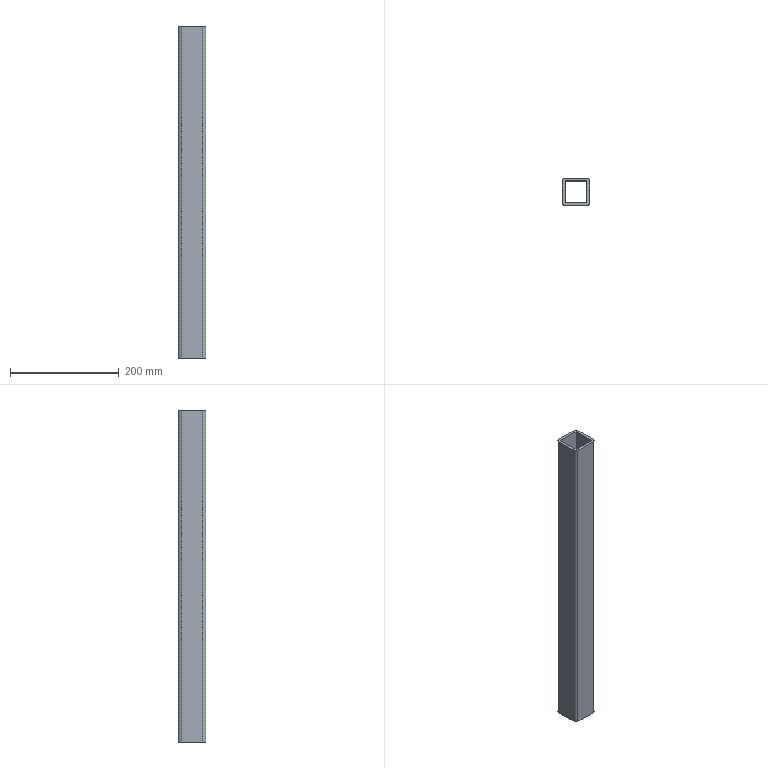Part | STEP file | SOLID | 1 solid | 14 faces | box 50 x 50 x 610 mm | volume 535909 mm3 | plane 10 | cylinder 4 | commonest cylinder face diameters 10 x4
STEP:
#1=CARTESIAN_POINT('',(0.,0.,0.));
#2=DIRECTION('',(0.,0.,1.));
#3=DIRECTION('',(1.,0.,0.));
#4=AXIS2_PLACEMENT_3D('',#1,#2,#3);
#5=CARTESIAN_POINT('',(-163.5,375.,-680.));
#6=VERTEX_POINT('',#5);
#7=CARTESIAN_POINT('',(-163.5,415.,-680.));
#8=VERTEX_POINT('',#7);
#9=CARTESIAN_POINT('',(-163.5,415.,-680.));
#10=DIRECTION('',(0.,1.,0.));
#11=VECTOR('',#10,1.);
#12=LINE('',#9,#11);
#13=CARTESIAN_POINT('',(-163.5,415.,430.));
#14=DIRECTION('',(-1.,0.,0.));
#15=DIRECTION('',(0.,1.,0.));
#16=AXIS2_PLACEMENT_3D('',#13,#14,#15);
#17=PLANE('',#16);
#18=CARTESIAN_POINT('',(0.,1110.));
#19=DIRECTION('',(1.,0.));
#20=VECTOR('',#19,1.);
#21=LINE('',#18,#20);
#22=(GEOMETRIC_REPRESENTATION_CONTEXT(2)PARAMETRIC_REPRESENTATION_CONTEXT()REPRESENTATION_CONTEXT('',''));
#23=DEFINITIONAL_REPRESENTATION('',(#21),#22);
#24=PCURVE('',#17,#23);
#25=CARTESIAN_POINT('',(-408.5,415.,-680.));
#26=DIRECTION('',(0.,0.,-1.));
#27=DIRECTION('',(0.,1.,0.));
#28=AXIS2_PLACEMENT_3D('',#25,#26,#27);
#29=PLANE('',#28);
#30=CARTESIAN_POINT('',(0.,245.));
#31=DIRECTION('',(1.,0.));
#32=VECTOR('',#31,1.);
#33=LINE('',#30,#32);
#34=(GEOMETRIC_REPRESENTATION_CONTEXT(2)PARAMETRIC_REPRESENTATION_CONTEXT()REPRESENTATION_CONTEXT('',''));
#35=DEFINITIONAL_REPRESENTATION('',(#33),#34);
#36=PCURVE('',#29,#35);
#37=SURFACE_CURVE('',#12,(#24,#36),.PCURVE_S1.);
#38=EDGE_CURVE('',#6,#8,#37,.T.);
#39=ORIENTED_EDGE('',*,*,#38,.F.);
#40=CARTESIAN_POINT('',(-163.5,375.,-70.));
#41=VERTEX_POINT('',#40);
#42=CARTESIAN_POINT('',(-163.5,375.,430.));
#43=DIRECTION('',(0.,0.,1.));
#44=VECTOR('',#43,1.);
#45=LINE('',#42,#44);
#46=CARTESIAN_POINT('',(-40.,0.));
#47=DIRECTION('',(0.,-1.));
#48=VECTOR('',#47,1.);
#49=LINE('',#46,#48);
#50=(GEOMETRIC_REPRESENTATION_CONTEXT(2)PARAMETRIC_REPRESENTATION_CONTEXT()REPRESENTATION_CONTEXT('',''));
#51=DEFINITIONAL_REPRESENTATION('',(#49),#50);
#52=PCURVE('',#17,#51);
#53=CARTESIAN_POINT('',(-163.5,375.,430.));
#54=DIRECTION('',(0.,1.,0.));
#55=DIRECTION('',(1.,0.,0.));
#56=AXIS2_PLACEMENT_3D('',#53,#54,#55);
#57=PLANE('',#56);
#58=CARTESIAN_POINT('',(0.,0.));
#59=DIRECTION('',(0.,-1.));
#60=VECTOR('',#59,1.);
#61=LINE('',#58,#60);
#62=(GEOMETRIC_REPRESENTATION_CONTEXT(2)PARAMETRIC_REPRESENTATION_CONTEXT()REPRESENTATION_CONTEXT('',''));
#63=DEFINITIONAL_REPRESENTATION('',(#61),#62);
#64=PCURVE('',#57,#63);
#65=SURFACE_CURVE('',#45,(#52,#64),.PCURVE_S1.);
#66=EDGE_CURVE('',#6,#41,#65,.T.);
#67=ORIENTED_EDGE('',*,*,#66,.T.);
#68=CARTESIAN_POINT('',(-163.5,415.,-70.));
#69=VERTEX_POINT('',#68);
#70=CARTESIAN_POINT('',(-163.5,415.,-70.));
#71=DIRECTION('',(0.,1.,0.));
#72=VECTOR('',#71,1.);
#73=LINE('',#70,#72);
#74=CARTESIAN_POINT('',(0.,500.));
#75=DIRECTION('',(1.,0.));
#76=VECTOR('',#75,1.);
#77=LINE('',#74,#76);
#78=(GEOMETRIC_REPRESENTATION_CONTEXT(2)PARAMETRIC_REPRESENTATION_CONTEXT()REPRESENTATION_CONTEXT('',''));
#79=DEFINITIONAL_REPRESENTATION('',(#77),#78);
#80=PCURVE('',#17,#79);
#81=CARTESIAN_POINT('',(-408.5,415.,-70.));
#82=DIRECTION('',(0.,0.,1.));
#83=DIRECTION('',(0.,1.,0.));
#84=AXIS2_PLACEMENT_3D('',#81,#82,#83);
#85=PLANE('',#84);
#86=CARTESIAN_POINT('',(0.,-245.));
#87=DIRECTION('',(1.,0.));
#88=VECTOR('',#87,1.);
#89=LINE('',#86,#88);
#90=(GEOMETRIC_REPRESENTATION_CONTEXT(2)PARAMETRIC_REPRESENTATION_CONTEXT()REPRESENTATION_CONTEXT('',''));
#91=DEFINITIONAL_REPRESENTATION('',(#89),#90);
#92=PCURVE('',#85,#91);
#93=SURFACE_CURVE('',#73,(#80,#92),.PCURVE_S1.);
#94=EDGE_CURVE('',#41,#69,#93,.T.);
#95=ORIENTED_EDGE('',*,*,#94,.T.);
#96=CARTESIAN_POINT('',(-163.5,415.,430.));
#97=DIRECTION('',(0.,0.,1.));
#98=VECTOR('',#97,1.);
#99=LINE('',#96,#98);
#100=CARTESIAN_POINT('',(0.,0.));
#101=DIRECTION('',(0.,-1.));
#102=VECTOR('',#101,1.);
#103=LINE('',#100,#102);
#104=(GEOMETRIC_REPRESENTATION_CONTEXT(2)PARAMETRIC_REPRESENTATION_CONTEXT()REPRESENTATION_CONTEXT('',''));
#105=DEFINITIONAL_REPRESENTATION('',(#103),#104);
#106=PCURVE('',#17,#105);
#107=CARTESIAN_POINT('',(-203.5,415.,430.));
#108=DIRECTION('',(0.,-1.,0.));
#109=DIRECTION('',(-1.,0.,0.));
#110=AXIS2_PLACEMENT_3D('',#107,#108,#109);
#111=PLANE('',#110);
#112=CARTESIAN_POINT('',(-40.,0.));
#113=DIRECTION('',(0.,-1.));
#114=VECTOR('',#113,1.);
#115=LINE('',#112,#114);
#116=(GEOMETRIC_REPRESENTATION_CONTEXT(2)PARAMETRIC_REPRESENTATION_CONTEXT()REPRESENTATION_CONTEXT('',''));
#117=DEFINITIONAL_REPRESENTATION('',(#115),#116);
#118=PCURVE('',#111,#117);
#119=SURFACE_CURVE('',#99,(#106,#118),.PCURVE_S1.);
#120=EDGE_CURVE('',#8,#69,#119,.T.);
#121=ORIENTED_EDGE('',*,*,#120,.F.);
#122=EDGE_LOOP('',(#39,#67,#95,#121));
#123=FACE_BOUND('',#122,.T.);
#124=ADVANCED_FACE('',(#123),#17,.T.);
#125=CARTESIAN_POINT('',(-203.5,375.,-680.));
#126=VERTEX_POINT('',#125);
#127=CARTESIAN_POINT('',(-408.5,375.,-680.));
#128=DIRECTION('',(1.,0.,0.));
#129=VECTOR('',#128,1.);
#130=LINE('',#127,#129);
#131=CARTESIAN_POINT('',(-245.,1110.));
#132=DIRECTION('',(1.,0.));
#133=VECTOR('',#132,1.);
#134=LINE('',#131,#133);
#135=(GEOMETRIC_REPRESENTATION_CONTEXT(2)PARAMETRIC_REPRESENTATION_CONTEXT()REPRESENTATION_CONTEXT('',''));
#136=DEFINITIONAL_REPRESENTATION('',(#134),#135);
#137=PCURVE('',#57,#136);
#138=CARTESIAN_POINT('',(-40.,0.));
#139=DIRECTION('',(0.,1.));
#140=VECTOR('',#139,1.);
#141=LINE('',#138,#140);
#142=(GEOMETRIC_REPRESENTATION_CONTEXT(2)PARAMETRIC_REPRESENTATION_CONTEXT()REPRESENTATION_CONTEXT('',''));
#143=DEFINITIONAL_REPRESENTATION('',(#141),#142);
#144=PCURVE('',#29,#143);
#145=SURFACE_CURVE('',#130,(#137,#144),.PCURVE_S1.);
#146=EDGE_CURVE('',#126,#6,#145,.T.);
#147=ORIENTED_EDGE('',*,*,#146,.F.);
#148=CARTESIAN_POINT('',(-203.5,375.,-70.));
#149=VERTEX_POINT('',#148);
#150=CARTESIAN_POINT('',(-203.5,375.,430.));
#151=DIRECTION('',(0.,0.,1.));
#152=VECTOR('',#151,1.);
#153=LINE('',#150,#152);
#154=CARTESIAN_POINT('',(-40.,0.));
#155=DIRECTION('',(0.,-1.));
#156=VECTOR('',#155,1.);
#157=LINE('',#154,#156);
#158=(GEOMETRIC_REPRESENTATION_CONTEXT(2)PARAMETRIC_REPRESENTATION_CONTEXT()REPRESENTATION_CONTEXT('',''));
#159=DEFINITIONAL_REPRESENTATION('',(#157),#158);
#160=PCURVE('',#57,#159);
#161=CARTESIAN_POINT('',(-203.5,375.,430.));
#162=DIRECTION('',(1.,0.,0.));
#163=DIRECTION('',(0.,-1.,0.));
#164=AXIS2_PLACEMENT_3D('',#161,#162,#163);
#165=PLANE('',#164);
#166=CARTESIAN_POINT('',(0.,0.));
#167=DIRECTION('',(0.,-1.));
#168=VECTOR('',#167,1.);
#169=LINE('',#166,#168);
#170=(GEOMETRIC_REPRESENTATION_CONTEXT(2)PARAMETRIC_REPRESENTATION_CONTEXT()REPRESENTATION_CONTEXT('',''));
#171=DEFINITIONAL_REPRESENTATION('',(#169),#170);
#172=PCURVE('',#165,#171);
#173=SURFACE_CURVE('',#153,(#160,#172),.PCURVE_S1.);
#174=EDGE_CURVE('',#126,#149,#173,.T.);
#175=ORIENTED_EDGE('',*,*,#174,.T.);
#176=CARTESIAN_POINT('',(-408.5,375.,-70.));
#177=DIRECTION('',(1.,0.,0.));
#178=VECTOR('',#177,1.);
#179=LINE('',#176,#178);
#180=CARTESIAN_POINT('',(-245.,500.));
#181=DIRECTION('',(1.,0.));
#182=VECTOR('',#181,1.);
#183=LINE('',#180,#182);
#184=(GEOMETRIC_REPRESENTATION_CONTEXT(2)PARAMETRIC_REPRESENTATION_CONTEXT()REPRESENTATION_CONTEXT('',''));
#185=DEFINITIONAL_REPRESENTATION('',(#183),#184);
#186=PCURVE('',#57,#185);
#187=CARTESIAN_POINT('',(-40.,0.));
#188=DIRECTION('',(0.,-1.));
#189=VECTOR('',#188,1.);
#190=LINE('',#187,#189);
#191=(GEOMETRIC_REPRESENTATION_CONTEXT(2)PARAMETRIC_REPRESENTATION_CONTEXT()REPRESENTATION_CONTEXT('',''));
#192=DEFINITIONAL_REPRESENTATION('',(#190),#191);
#193=PCURVE('',#85,#192);
#194=SURFACE_CURVE('',#179,(#186,#193),.PCURVE_S1.);
#195=EDGE_CURVE('',#149,#41,#194,.T.);
#196=ORIENTED_EDGE('',*,*,#195,.T.);
#197=ORIENTED_EDGE('',*,*,#66,.F.);
#198=EDGE_LOOP('',(#147,#175,#196,#197));
#199=FACE_BOUND('',#198,.T.);
#200=ADVANCED_FACE('',(#199),#57,.T.);
#201=CARTESIAN_POINT('',(-203.5,415.,-680.));
#202=VERTEX_POINT('',#201);
#203=CARTESIAN_POINT('',(-203.5,415.,-680.));
#204=DIRECTION('',(0.,-1.,0.));
#205=VECTOR('',#204,1.);
#206=LINE('',#203,#205);
#207=CARTESIAN_POINT('',(-40.,1110.));
#208=DIRECTION('',(1.,0.));
#209=VECTOR('',#208,1.);
#210=LINE('',#207,#209);
#211=(GEOMETRIC_REPRESENTATION_CONTEXT(2)PARAMETRIC_REPRESENTATION_CONTEXT()REPRESENTATION_CONTEXT('',''));
#212=DEFINITIONAL_REPRESENTATION('',(#210),#211);
#213=PCURVE('',#165,#212);
#214=CARTESIAN_POINT('',(0.,205.));
#215=DIRECTION('',(-1.,0.));
#216=VECTOR('',#215,1.);
#217=LINE('',#214,#216);
#218=(GEOMETRIC_REPRESENTATION_CONTEXT(2)PARAMETRIC_REPRESENTATION_CONTEXT()REPRESENTATION_CONTEXT('',''));
#219=DEFINITIONAL_REPRESENTATION('',(#217),#218);
#220=PCURVE('',#29,#219);
#221=SURFACE_CURVE('',#206,(#213,#220),.PCURVE_S1.);
#222=EDGE_CURVE('',#202,#126,#221,.T.);
#223=ORIENTED_EDGE('',*,*,#222,.F.);
#224=CARTESIAN_POINT('',(-203.5,415.,-70.));
#225=VERTEX_POINT('',#224);
#226=CARTESIAN_POINT('',(-203.5,415.,430.));
#227=DIRECTION('',(0.,0.,1.));
#228=VECTOR('',#227,1.);
#229=LINE('',#226,#228);
#230=CARTESIAN_POINT('',(-40.,0.));
#231=DIRECTION('',(0.,-1.));
#232=VECTOR('',#231,1.);
#233=LINE('',#230,#232);
#234=(GEOMETRIC_REPRESENTATION_CONTEXT(2)PARAMETRIC_REPRESENTATION_CONTEXT()REPRESENTATION_CONTEXT('',''));
#235=DEFINITIONAL_REPRESENTATION('',(#233),#234);
#236=PCURVE('',#165,#235);
#237=CARTESIAN_POINT('',(0.,0.));
#238=DIRECTION('',(0.,-1.));
#239=VECTOR('',#238,1.);
#240=LINE('',#237,#239);
#241=(GEOMETRIC_REPRESENTATION_CONTEXT(2)PARAMETRIC_REPRESENTATION_CONTEXT()REPRESENTATION_CONTEXT('',''));
#242=DEFINITIONAL_REPRESENTATION('',(#240),#241);
#243=PCURVE('',#111,#242);
#244=SURFACE_CURVE('',#229,(#236,#243),.PCURVE_S1.);
#245=EDGE_CURVE('',#202,#225,#244,.T.);
#246=ORIENTED_EDGE('',*,*,#245,.T.);
#247=CARTESIAN_POINT('',(-203.5,415.,-70.));
#248=DIRECTION('',(0.,-1.,0.));
#249=VECTOR('',#248,1.);
#250=LINE('',#247,#249);
#251=CARTESIAN_POINT('',(-40.,500.));
#252=DIRECTION('',(1.,0.));
#253=VECTOR('',#252,1.);
#254=LINE('',#251,#253);
#255=(GEOMETRIC_REPRESENTATION_CONTEXT(2)PARAMETRIC_REPRESENTATION_CONTEXT()REPRESENTATION_CONTEXT('',''));
#256=DEFINITIONAL_REPRESENTATION('',(#254),#255);
#257=PCURVE('',#165,#256);
#258=CARTESIAN_POINT('',(0.,-205.));
#259=DIRECTION('',(-1.,0.));
#260=VECTOR('',#259,1.);
#261=LINE('',#258,#260);
#262=(GEOMETRIC_REPRESENTATION_CONTEXT(2)PARAMETRIC_REPRESENTATION_CONTEXT()REPRESENTATION_CONTEXT('',''));
#263=DEFINITIONAL_REPRESENTATION('',(#261),#262);
#264=PCURVE('',#85,#263);
#265=SURFACE_CURVE('',#250,(#257,#264),.PCURVE_S1.);
#266=EDGE_CURVE('',#225,#149,#265,.T.);
#267=ORIENTED_EDGE('',*,*,#266,.T.);
#268=ORIENTED_EDGE('',*,*,#174,.F.);
#269=EDGE_LOOP('',(#223,#246,#267,#268));
#270=FACE_BOUND('',#269,.T.);
#271=ADVANCED_FACE('',(#270),#165,.T.);
#272=CARTESIAN_POINT('',(-158.5,415.,-680.));
#273=VERTEX_POINT('',#272);
#274=CARTESIAN_POINT('',(-158.5,375.,-680.));
#275=VERTEX_POINT('',#274);
#276=CARTESIAN_POINT('',(-158.5,415.,-680.));
#277=DIRECTION('',(0.,-1.,0.));
#278=VECTOR('',#277,1.);
#279=LINE('',#276,#278);
#280=CARTESIAN_POINT('',(-158.5,375.,430.));
#281=DIRECTION('',(1.,0.,0.));
#282=DIRECTION('',(0.,-1.,0.));
#283=AXIS2_PLACEMENT_3D('',#280,#281,#282);
#284=PLANE('',#283);
#285=CARTESIAN_POINT('',(-40.,1110.));
#286=DIRECTION('',(1.,0.));
#287=VECTOR('',#286,1.);
#288=LINE('',#285,#287);
#289=(GEOMETRIC_REPRESENTATION_CONTEXT(2)PARAMETRIC_REPRESENTATION_CONTEXT()REPRESENTATION_CONTEXT('',''));
#290=DEFINITIONAL_REPRESENTATION('',(#288),#289);
#291=PCURVE('',#284,#290);
#292=CARTESIAN_POINT('',(0.,250.));
#293=DIRECTION('',(-1.,0.));
#294=VECTOR('',#293,1.);
#295=LINE('',#292,#294);
#296=(GEOMETRIC_REPRESENTATION_CONTEXT(2)PARAMETRIC_REPRESENTATION_CONTEXT()REPRESENTATION_CONTEXT('',''));
#297=DEFINITIONAL_REPRESENTATION('',(#295),#296);
#298=PCURVE('',#29,#297);
#299=SURFACE_CURVE('',#279,(#291,#298),.PCURVE_S1.);
#300=EDGE_CURVE('',#273,#275,#299,.T.);
#301=ORIENTED_EDGE('',*,*,#300,.F.);
#302=CARTESIAN_POINT('',(-158.5,415.,-70.));
#303=VERTEX_POINT('',#302);
#304=CARTESIAN_POINT('',(-158.5,415.,430.));
#305=DIRECTION('',(0.,0.,1.));
#306=VECTOR('',#305,1.);
#307=LINE('',#304,#306);
#308=CARTESIAN_POINT('',(-40.,0.));
#309=DIRECTION('',(0.,-1.));
#310=VECTOR('',#309,1.);
#311=LINE('',#308,#310);
#312=(GEOMETRIC_REPRESENTATION_CONTEXT(2)PARAMETRIC_REPRESENTATION_CONTEXT()REPRESENTATION_CONTEXT('',''));
#313=DEFINITIONAL_REPRESENTATION('',(#311),#312);
#314=PCURVE('',#284,#313);
#315=CARTESIAN_POINT('',(-163.5,415.,430.));
#316=DIRECTION('',(0.,0.,-1.));
#317=DIRECTION('',(0.,1.,0.));
#318=AXIS2_PLACEMENT_3D('',#315,#316,#317);
#319=CYLINDRICAL_SURFACE('',#318,5.);
#320=CARTESIAN_POINT('',(1.571,0.));
#321=DIRECTION('',(0.,-1.));
#322=VECTOR('',#321,1.);
#323=LINE('',#320,#322);
#324=(GEOMETRIC_REPRESENTATION_CONTEXT(2)PARAMETRIC_REPRESENTATION_CONTEXT()REPRESENTATION_CONTEXT('',''));
#325=DEFINITIONAL_REPRESENTATION('',(#323),#324);
#326=PCURVE('',#319,#325);
#327=SURFACE_CURVE('',#307,(#314,#326),.PCURVE_S1.);
#328=EDGE_CURVE('',#273,#303,#327,.T.);
#329=ORIENTED_EDGE('',*,*,#328,.T.);
#330=CARTESIAN_POINT('',(-158.5,375.,-70.));
#331=VERTEX_POINT('',#330);
#332=CARTESIAN_POINT('',(-158.5,415.,-70.));
#333=DIRECTION('',(0.,-1.,0.));
#334=VECTOR('',#333,1.);
#335=LINE('',#332,#334);
#336=CARTESIAN_POINT('',(-40.,500.));
#337=DIRECTION('',(1.,0.));
#338=VECTOR('',#337,1.);
#339=LINE('',#336,#338);
#340=(GEOMETRIC_REPRESENTATION_CONTEXT(2)PARAMETRIC_REPRESENTATION_CONTEXT()REPRESENTATION_CONTEXT('',''));
#341=DEFINITIONAL_REPRESENTATION('',(#339),#340);
#342=PCURVE('',#284,#341);
#343=CARTESIAN_POINT('',(0.,-250.));
#344=DIRECTION('',(-1.,0.));
#345=VECTOR('',#344,1.);
#346=LINE('',#343,#345);
#347=(GEOMETRIC_REPRESENTATION_CONTEXT(2)PARAMETRIC_REPRESENTATION_CONTEXT()REPRESENTATION_CONTEXT('',''));
#348=DEFINITIONAL_REPRESENTATION('',(#346),#347);
#349=PCURVE('',#85,#348);
#350=SURFACE_CURVE('',#335,(#342,#349),.PCURVE_S1.);
#351=EDGE_CURVE('',#303,#331,#350,.T.);
#352=ORIENTED_EDGE('',*,*,#351,.T.);
#353=CARTESIAN_POINT('',(-158.5,375.,430.));
#354=DIRECTION('',(0.,0.,1.));
#355=VECTOR('',#354,1.);
#356=LINE('',#353,#355);
#357=CARTESIAN_POINT('',(0.,0.));
#358=DIRECTION('',(0.,-1.));
#359=VECTOR('',#358,1.);
#360=LINE('',#357,#359);
#361=(GEOMETRIC_REPRESENTATION_CONTEXT(2)PARAMETRIC_REPRESENTATION_CONTEXT()REPRESENTATION_CONTEXT('',''));
#362=DEFINITIONAL_REPRESENTATION('',(#360),#361);
#363=PCURVE('',#284,#362);
#364=CARTESIAN_POINT('',(-163.5,375.,430.));
#365=DIRECTION('',(0.,0.,-1.));
#366=DIRECTION('',(0.,1.,0.));
#367=AXIS2_PLACEMENT_3D('',#364,#365,#366);
#368=CYLINDRICAL_SURFACE('',#367,5.);
#369=CARTESIAN_POINT('',(1.571,0.));
#370=DIRECTION('',(0.,-1.));
#371=VECTOR('',#370,1.);
#372=LINE('',#369,#371);
#373=(GEOMETRIC_REPRESENTATION_CONTEXT(2)PARAMETRIC_REPRESENTATION_CONTEXT()REPRESENTATION_CONTEXT('',''));
#374=DEFINITIONAL_REPRESENTATION('',(#372),#373);
#375=PCURVE('',#368,#374);
#376=SURFACE_CURVE('',#356,(#363,#375),.PCURVE_S1.);
#377=EDGE_CURVE('',#275,#331,#376,.T.);
#378=ORIENTED_EDGE('',*,*,#377,.F.);
#379=EDGE_LOOP('',(#301,#329,#352,#378));
#380=FACE_BOUND('',#379,.T.);
#381=ADVANCED_FACE('',(#380),#284,.T.);
#382=CARTESIAN_POINT('',(-163.5,420.,-680.));
#383=VERTEX_POINT('',#382);
#384=CARTESIAN_POINT('',(-163.5,415.,-680.));
#385=DIRECTION('',(0.,0.,-1.));
#386=DIRECTION('',(0.,1.,0.));
#387=AXIS2_PLACEMENT_3D('',#384,#385,#386);
#388=CIRCLE('',#387,5.);
#389=CARTESIAN_POINT('',(0.,1110.));
#390=DIRECTION('',(1.,0.));
#391=VECTOR('',#390,1.);
#392=LINE('',#389,#391);
#393=(GEOMETRIC_REPRESENTATION_CONTEXT(2)PARAMETRIC_REPRESENTATION_CONTEXT()REPRESENTATION_CONTEXT('',''));
#394=DEFINITIONAL_REPRESENTATION('',(#392),#393);
#395=PCURVE('',#319,#394);
#396=CARTESIAN_POINT('',(0.,245.));
#397=DIRECTION('',(1.,0.));
#398=AXIS2_PLACEMENT_2D('',#396,#397);
#399=CIRCLE('',#398,5.);
#400=(GEOMETRIC_REPRESENTATION_CONTEXT(2)PARAMETRIC_REPRESENTATION_CONTEXT()REPRESENTATION_CONTEXT('',''));
#401=DEFINITIONAL_REPRESENTATION('',(#399),#400);
#402=PCURVE('',#29,#401);
#403=SURFACE_CURVE('',#388,(#395,#402),.PCURVE_S1.);
#404=EDGE_CURVE('',#383,#273,#403,.T.);
#405=ORIENTED_EDGE('',*,*,#404,.F.);
#406=CARTESIAN_POINT('',(-163.5,420.,-70.));
#407=VERTEX_POINT('',#406);
#408=CARTESIAN_POINT('',(-163.5,420.,430.));
#409=DIRECTION('',(0.,0.,1.));
#410=VECTOR('',#409,1.);
#411=LINE('',#408,#410);
#412=CARTESIAN_POINT('',(0.,0.));
#413=DIRECTION('',(0.,-1.));
#414=VECTOR('',#413,1.);
#415=LINE('',#412,#414);
#416=(GEOMETRIC_REPRESENTATION_CONTEXT(2)PARAMETRIC_REPRESENTATION_CONTEXT()REPRESENTATION_CONTEXT('',''));
#417=DEFINITIONAL_REPRESENTATION('',(#415),#416);
#418=PCURVE('',#319,#417);
#419=CARTESIAN_POINT('',(-163.5,420.,430.));
#420=DIRECTION('',(0.,1.,0.));
#421=DIRECTION('',(1.,0.,0.));
#422=AXIS2_PLACEMENT_3D('',#419,#420,#421);
#423=PLANE('',#422);
#424=CARTESIAN_POINT('',(0.,0.));
#425=DIRECTION('',(0.,-1.));
#426=VECTOR('',#425,1.);
#427=LINE('',#424,#426);
#428=(GEOMETRIC_REPRESENTATION_CONTEXT(2)PARAMETRIC_REPRESENTATION_CONTEXT()REPRESENTATION_CONTEXT('',''));
#429=DEFINITIONAL_REPRESENTATION('',(#427),#428);
#430=PCURVE('',#423,#429);
#431=SURFACE_CURVE('',#411,(#418,#430),.PCURVE_S1.);
#432=EDGE_CURVE('',#383,#407,#431,.T.);
#433=ORIENTED_EDGE('',*,*,#432,.T.);
#434=CARTESIAN_POINT('',(-163.5,415.,-70.));
#435=DIRECTION('',(0.,0.,-1.));
#436=DIRECTION('',(0.,1.,0.));
#437=AXIS2_PLACEMENT_3D('',#434,#435,#436);
#438=CIRCLE('',#437,5.);
#439=CARTESIAN_POINT('',(0.,500.));
#440=DIRECTION('',(1.,0.));
#441=VECTOR('',#440,1.);
#442=LINE('',#439,#441);
#443=(GEOMETRIC_REPRESENTATION_CONTEXT(2)PARAMETRIC_REPRESENTATION_CONTEXT()REPRESENTATION_CONTEXT('',''));
#444=DEFINITIONAL_REPRESENTATION('',(#442),#443);
#445=PCURVE('',#319,#444);
#446=CARTESIAN_POINT('',(5.,-245.));
#447=CARTESIAN_POINT('',(5.,-253.66));
#448=CARTESIAN_POINT('',(-2.5,-249.33));
#449=CARTESIAN_POINT('',(-10.,-245.));
#450=CARTESIAN_POINT('',(-2.5,-240.67));
#451=CARTESIAN_POINT('',(5.,-236.34));
#452=CARTESIAN_POINT('',(5.,-245.));
#453=(BOUNDED_CURVE()B_SPLINE_CURVE(2,(#446,#447,#448,#449,#450,#451,#452),.UNSPECIFIED.,.T.,.F.)B_SPLINE_CURVE_WITH_KNOTS((1,2,2,2,2,1),(-2.094,0.,2.094,4.189,6.283,8.378),.UNSPECIFIED.)CURVE()GEOMETRIC_REPRESENTATION_ITEM()RATIONAL_B_SPLINE_CURVE((1.,0.5,1.,0.5,1.,0.5,1.))REPRESENTATION_ITEM(''));
#454=(GEOMETRIC_REPRESENTATION_CONTEXT(2)PARAMETRIC_REPRESENTATION_CONTEXT()REPRESENTATION_CONTEXT('',''));
#455=DEFINITIONAL_REPRESENTATION('',(#453),#454);
#456=PCURVE('',#85,#455);
#457=SURFACE_CURVE('',#438,(#445,#456),.PCURVE_S1.);
#458=EDGE_CURVE('',#407,#303,#457,.T.);
#459=ORIENTED_EDGE('',*,*,#458,.T.);
#460=ORIENTED_EDGE('',*,*,#328,.F.);
#461=EDGE_LOOP('',(#405,#433,#459,#460));
#462=FACE_BOUND('',#461,.T.);
#463=ADVANCED_FACE('',(#462),#319,.T.);
#464=CARTESIAN_POINT('',(-203.5,420.,-680.));
#465=VERTEX_POINT('',#464);
#466=CARTESIAN_POINT('',(-408.5,420.,-680.));
#467=DIRECTION('',(1.,0.,0.));
#468=VECTOR('',#467,1.);
#469=LINE('',#466,#468);
#470=CARTESIAN_POINT('',(-245.,1110.));
#471=DIRECTION('',(1.,0.));
#472=VECTOR('',#471,1.);
#473=LINE('',#470,#472);
#474=(GEOMETRIC_REPRESENTATION_CONTEXT(2)PARAMETRIC_REPRESENTATION_CONTEXT()REPRESENTATION_CONTEXT('',''));
#475=DEFINITIONAL_REPRESENTATION('',(#473),#474);
#476=PCURVE('',#423,#475);
#477=CARTESIAN_POINT('',(5.,0.));
#478=DIRECTION('',(0.,1.));
#479=VECTOR('',#478,1.);
#480=LINE('',#477,#479);
#481=(GEOMETRIC_REPRESENTATION_CONTEXT(2)PARAMETRIC_REPRESENTATION_CONTEXT()REPRESENTATION_CONTEXT('',''));
#482=DEFINITIONAL_REPRESENTATION('',(#480),#481);
#483=PCURVE('',#29,#482);
#484=SURFACE_CURVE('',#469,(#476,#483),.PCURVE_S1.);
#485=EDGE_CURVE('',#465,#383,#484,.T.);
#486=ORIENTED_EDGE('',*,*,#485,.F.);
#487=CARTESIAN_POINT('',(-203.5,420.,-70.));
#488=VERTEX_POINT('',#487);
#489=CARTESIAN_POINT('',(-203.5,420.,430.));
#490=DIRECTION('',(0.,0.,1.));
#491=VECTOR('',#490,1.);
#492=LINE('',#489,#491);
#493=CARTESIAN_POINT('',(-40.,0.));
#494=DIRECTION('',(0.,-1.));
#495=VECTOR('',#494,1.);
#496=LINE('',#493,#495);
#497=(GEOMETRIC_REPRESENTATION_CONTEXT(2)PARAMETRIC_REPRESENTATION_CONTEXT()REPRESENTATION_CONTEXT('',''));
#498=DEFINITIONAL_REPRESENTATION('',(#496),#497);
#499=PCURVE('',#423,#498);
#500=CARTESIAN_POINT('',(-203.5,415.,430.));
#501=DIRECTION('',(0.,0.,-1.));
#502=DIRECTION('',(0.,1.,0.));
#503=AXIS2_PLACEMENT_3D('',#500,#501,#502);
#504=CYLINDRICAL_SURFACE('',#503,5.);
#505=CARTESIAN_POINT('',(6.283,0.));
#506=DIRECTION('',(0.,-1.));
#507=VECTOR('',#506,1.);
#508=LINE('',#505,#507);
#509=(GEOMETRIC_REPRESENTATION_CONTEXT(2)PARAMETRIC_REPRESENTATION_CONTEXT()REPRESENTATION_CONTEXT('',''));
#510=DEFINITIONAL_REPRESENTATION('',(#508),#509);
#511=PCURVE('',#504,#510);
#512=SURFACE_CURVE('',#492,(#499,#511),.PCURVE_S1.);
#513=EDGE_CURVE('',#465,#488,#512,.T.);
#514=ORIENTED_EDGE('',*,*,#513,.T.);
#515=CARTESIAN_POINT('',(-408.5,420.,-70.));
#516=DIRECTION('',(1.,0.,0.));
#517=VECTOR('',#516,1.);
#518=LINE('',#515,#517);
#519=CARTESIAN_POINT('',(-245.,500.));
#520=DIRECTION('',(1.,0.));
#521=VECTOR('',#520,1.);
#522=LINE('',#519,#521);
#523=(GEOMETRIC_REPRESENTATION_CONTEXT(2)PARAMETRIC_REPRESENTATION_CONTEXT()REPRESENTATION_CONTEXT('',''));
#524=DEFINITIONAL_REPRESENTATION('',(#522),#523);
#525=PCURVE('',#423,#524);
#526=CARTESIAN_POINT('',(5.,0.));
#527=DIRECTION('',(0.,-1.));
#528=VECTOR('',#527,1.);
#529=LINE('',#526,#528);
#530=(GEOMETRIC_REPRESENTATION_CONTEXT(2)PARAMETRIC_REPRESENTATION_CONTEXT()REPRESENTATION_CONTEXT('',''));
#531=DEFINITIONAL_REPRESENTATION('',(#529),#530);
#532=PCURVE('',#85,#531);
#533=SURFACE_CURVE('',#518,(#525,#532),.PCURVE_S1.);
#534=EDGE_CURVE('',#488,#407,#533,.T.);
#535=ORIENTED_EDGE('',*,*,#534,.T.);
#536=ORIENTED_EDGE('',*,*,#432,.F.);
#537=EDGE_LOOP('',(#486,#514,#535,#536));
#538=FACE_BOUND('',#537,.T.);
#539=ADVANCED_FACE('',(#538),#423,.T.);
#540=CARTESIAN_POINT('',(-208.5,415.,-680.));
#541=VERTEX_POINT('',#540);
#542=CARTESIAN_POINT('',(-203.5,415.,-680.));
#543=DIRECTION('',(0.,0.,-1.));
#544=DIRECTION('',(0.,1.,0.));
#545=AXIS2_PLACEMENT_3D('',#542,#543,#544);
#546=CIRCLE('',#545,5.);
#547=CARTESIAN_POINT('',(0.,1110.));
#548=DIRECTION('',(1.,0.));
#549=VECTOR('',#548,1.);
#550=LINE('',#547,#549);
#551=(GEOMETRIC_REPRESENTATION_CONTEXT(2)PARAMETRIC_REPRESENTATION_CONTEXT()REPRESENTATION_CONTEXT('',''));
#552=DEFINITIONAL_REPRESENTATION('',(#550),#551);
#553=PCURVE('',#504,#552);
#554=CARTESIAN_POINT('',(0.,205.));
#555=DIRECTION('',(1.,0.));
#556=AXIS2_PLACEMENT_2D('',#554,#555);
#557=CIRCLE('',#556,5.);
#558=(GEOMETRIC_REPRESENTATION_CONTEXT(2)PARAMETRIC_REPRESENTATION_CONTEXT()REPRESENTATION_CONTEXT('',''));
#559=DEFINITIONAL_REPRESENTATION('',(#557),#558);
#560=PCURVE('',#29,#559);
#561=SURFACE_CURVE('',#546,(#553,#560),.PCURVE_S1.);
#562=EDGE_CURVE('',#541,#465,#561,.T.);
#563=ORIENTED_EDGE('',*,*,#562,.F.);
#564=CARTESIAN_POINT('',(-208.5,415.,-70.));
#565=VERTEX_POINT('',#564);
#566=CARTESIAN_POINT('',(-208.5,415.,430.));
#567=DIRECTION('',(0.,0.,1.));
#568=VECTOR('',#567,1.);
#569=LINE('',#566,#568);
#570=CARTESIAN_POINT('',(4.712,0.));
#571=DIRECTION('',(0.,-1.));
#572=VECTOR('',#571,1.);
#573=LINE('',#570,#572);
#574=(GEOMETRIC_REPRESENTATION_CONTEXT(2)PARAMETRIC_REPRESENTATION_CONTEXT()REPRESENTATION_CONTEXT('',''));
#575=DEFINITIONAL_REPRESENTATION('',(#573),#574);
#576=PCURVE('',#504,#575);
#577=CARTESIAN_POINT('',(-208.5,415.,430.));
#578=DIRECTION('',(-1.,0.,0.));
#579=DIRECTION('',(0.,1.,0.));
#580=AXIS2_PLACEMENT_3D('',#577,#578,#579);
#581=PLANE('',#580);
#582=CARTESIAN_POINT('',(0.,0.));
#583=DIRECTION('',(0.,-1.));
#584=VECTOR('',#583,1.);
#585=LINE('',#582,#584);
#586=(GEOMETRIC_REPRESENTATION_CONTEXT(2)PARAMETRIC_REPRESENTATION_CONTEXT()REPRESENTATION_CONTEXT('',''));
#587=DEFINITIONAL_REPRESENTATION('',(#585),#586);
#588=PCURVE('',#581,#587);
#589=SURFACE_CURVE('',#569,(#576,#588),.PCURVE_S1.);
#590=EDGE_CURVE('',#541,#565,#589,.T.);
#591=ORIENTED_EDGE('',*,*,#590,.T.);
#592=CARTESIAN_POINT('',(-203.5,415.,-70.));
#593=DIRECTION('',(0.,0.,-1.));
#594=DIRECTION('',(0.,1.,0.));
#595=AXIS2_PLACEMENT_3D('',#592,#593,#594);
#596=CIRCLE('',#595,5.);
#597=CARTESIAN_POINT('',(0.,500.));
#598=DIRECTION('',(1.,0.));
#599=VECTOR('',#598,1.);
#600=LINE('',#597,#599);
#601=(GEOMETRIC_REPRESENTATION_CONTEXT(2)PARAMETRIC_REPRESENTATION_CONTEXT()REPRESENTATION_CONTEXT('',''));
#602=DEFINITIONAL_REPRESENTATION('',(#600),#601);
#603=PCURVE('',#504,#602);
#604=CARTESIAN_POINT('',(5.,-205.));
#605=CARTESIAN_POINT('',(5.,-213.66));
#606=CARTESIAN_POINT('',(-2.5,-209.33));
#607=CARTESIAN_POINT('',(-10.,-205.));
#608=CARTESIAN_POINT('',(-2.5,-200.67));
#609=CARTESIAN_POINT('',(5.,-196.34));
#610=CARTESIAN_POINT('',(5.,-205.));
#611=(BOUNDED_CURVE()B_SPLINE_CURVE(2,(#604,#605,#606,#607,#608,#609,#610),.UNSPECIFIED.,.T.,.F.)B_SPLINE_CURVE_WITH_KNOTS((1,2,2,2,2,1),(-2.094,0.,2.094,4.189,6.283,8.378),.UNSPECIFIED.)CURVE()GEOMETRIC_REPRESENTATION_ITEM()RATIONAL_B_SPLINE_CURVE((1.,0.5,1.,0.5,1.,0.5,1.))REPRESENTATION_ITEM(''));
#612=(GEOMETRIC_REPRESENTATION_CONTEXT(2)PARAMETRIC_REPRESENTATION_CONTEXT()REPRESENTATION_CONTEXT('',''));
#613=DEFINITIONAL_REPRESENTATION('',(#611),#612);
#614=PCURVE('',#85,#613);
#615=SURFACE_CURVE('',#596,(#603,#614),.PCURVE_S1.);
#616=EDGE_CURVE('',#565,#488,#615,.T.);
#617=ORIENTED_EDGE('',*,*,#616,.T.);
#618=ORIENTED_EDGE('',*,*,#513,.F.);
#619=EDGE_LOOP('',(#563,#591,#617,#618));
#620=FACE_BOUND('',#619,.T.);
#621=ADVANCED_FACE('',(#620),#504,.T.);
#622=CARTESIAN_POINT('',(-208.5,375.,-680.));
#623=VERTEX_POINT('',#622);
#624=CARTESIAN_POINT('',(-208.5,415.,-680.));
#625=DIRECTION('',(0.,1.,0.));
#626=VECTOR('',#625,1.);
#627=LINE('',#624,#626);
#628=CARTESIAN_POINT('',(0.,1110.));
#629=DIRECTION('',(1.,0.));
#630=VECTOR('',#629,1.);
#631=LINE('',#628,#630);
#632=(GEOMETRIC_REPRESENTATION_CONTEXT(2)PARAMETRIC_REPRESENTATION_CONTEXT()REPRESENTATION_CONTEXT('',''));
#633=DEFINITIONAL_REPRESENTATION('',(#631),#632);
#634=PCURVE('',#581,#633);
#635=CARTESIAN_POINT('',(0.,200.));
#636=DIRECTION('',(1.,0.));
#637=VECTOR('',#636,1.);
#638=LINE('',#635,#637);
#639=(GEOMETRIC_REPRESENTATION_CONTEXT(2)PARAMETRIC_REPRESENTATION_CONTEXT()REPRESENTATION_CONTEXT('',''));
#640=DEFINITIONAL_REPRESENTATION('',(#638),#639);
#641=PCURVE('',#29,#640);
#642=SURFACE_CURVE('',#627,(#634,#641),.PCURVE_S1.);
#643=EDGE_CURVE('',#623,#541,#642,.T.);
#644=ORIENTED_EDGE('',*,*,#643,.F.);
#645=CARTESIAN_POINT('',(-208.5,375.,-70.));
#646=VERTEX_POINT('',#645);
#647=CARTESIAN_POINT('',(-208.5,375.,430.));
#648=DIRECTION('',(0.,0.,1.));
#649=VECTOR('',#648,1.);
#650=LINE('',#647,#649);
#651=CARTESIAN_POINT('',(-40.,0.));
#652=DIRECTION('',(0.,-1.));
#653=VECTOR('',#652,1.);
#654=LINE('',#651,#653);
#655=(GEOMETRIC_REPRESENTATION_CONTEXT(2)PARAMETRIC_REPRESENTATION_CONTEXT()REPRESENTATION_CONTEXT('',''));
#656=DEFINITIONAL_REPRESENTATION('',(#654),#655);
#657=PCURVE('',#581,#656);
#658=CARTESIAN_POINT('',(-203.5,375.,430.));
#659=DIRECTION('',(0.,0.,-1.));
#660=DIRECTION('',(0.,1.,0.));
#661=AXIS2_PLACEMENT_3D('',#658,#659,#660);
#662=CYLINDRICAL_SURFACE('',#661,5.);
#663=CARTESIAN_POINT('',(4.712,0.));
#664=DIRECTION('',(0.,-1.));
#665=VECTOR('',#664,1.);
#666=LINE('',#663,#665);
#667=(GEOMETRIC_REPRESENTATION_CONTEXT(2)PARAMETRIC_REPRESENTATION_CONTEXT()REPRESENTATION_CONTEXT('',''));
#668=DEFINITIONAL_REPRESENTATION('',(#666),#667);
#669=PCURVE('',#662,#668);
#670=SURFACE_CURVE('',#650,(#657,#669),.PCURVE_S1.);
#671=EDGE_CURVE('',#623,#646,#670,.T.);
#672=ORIENTED_EDGE('',*,*,#671,.T.);
#673=CARTESIAN_POINT('',(-208.5,415.,-70.));
#674=DIRECTION('',(0.,1.,0.));
#675=VECTOR('',#674,1.);
#676=LINE('',#673,#675);
#677=CARTESIAN_POINT('',(0.,500.));
#678=DIRECTION('',(1.,0.));
#679=VECTOR('',#678,1.);
#680=LINE('',#677,#679);
#681=(GEOMETRIC_REPRESENTATION_CONTEXT(2)PARAMETRIC_REPRESENTATION_CONTEXT()REPRESENTATION_CONTEXT('',''));
#682=DEFINITIONAL_REPRESENTATION('',(#680),#681);
#683=PCURVE('',#581,#682);
#684=CARTESIAN_POINT('',(0.,-200.));
#685=DIRECTION('',(1.,0.));
#686=VECTOR('',#685,1.);
#687=LINE('',#684,#686);
#688=(GEOMETRIC_REPRESENTATION_CONTEXT(2)PARAMETRIC_REPRESENTATION_CONTEXT()REPRESENTATION_CONTEXT('',''));
#689=DEFINITIONAL_REPRESENTATION('',(#687),#688);
#690=PCURVE('',#85,#689);
#691=SURFACE_CURVE('',#676,(#683,#690),.PCURVE_S1.);
#692=EDGE_CURVE('',#646,#565,#691,.T.);
#693=ORIENTED_EDGE('',*,*,#692,.T.);
#694=ORIENTED_EDGE('',*,*,#590,.F.);
#695=EDGE_LOOP('',(#644,#672,#693,#694));
#696=FACE_BOUND('',#695,.T.);
#697=ADVANCED_FACE('',(#696),#581,.T.);
#698=CARTESIAN_POINT('',(-203.5,370.,-680.));
#699=VERTEX_POINT('',#698);
#700=CARTESIAN_POINT('',(-203.5,375.,-680.));
#701=DIRECTION('',(0.,0.,-1.));
#702=DIRECTION('',(0.,1.,0.));
#703=AXIS2_PLACEMENT_3D('',#700,#701,#702);
#704=CIRCLE('',#703,5.);
#705=CARTESIAN_POINT('',(0.,1110.));
#706=DIRECTION('',(1.,0.));
#707=VECTOR('',#706,1.);
#708=LINE('',#705,#707);
#709=(GEOMETRIC_REPRESENTATION_CONTEXT(2)PARAMETRIC_REPRESENTATION_CONTEXT()REPRESENTATION_CONTEXT('',''));
#710=DEFINITIONAL_REPRESENTATION('',(#708),#709);
#711=PCURVE('',#662,#710);
#712=CARTESIAN_POINT('',(-40.,205.));
#713=DIRECTION('',(1.,0.));
#714=AXIS2_PLACEMENT_2D('',#712,#713);
#715=CIRCLE('',#714,5.);
#716=(GEOMETRIC_REPRESENTATION_CONTEXT(2)PARAMETRIC_REPRESENTATION_CONTEXT()REPRESENTATION_CONTEXT('',''));
#717=DEFINITIONAL_REPRESENTATION('',(#715),#716);
#718=PCURVE('',#29,#717);
#719=SURFACE_CURVE('',#704,(#711,#718),.PCURVE_S1.);
#720=EDGE_CURVE('',#699,#623,#719,.T.);
#721=ORIENTED_EDGE('',*,*,#720,.F.);
#722=CARTESIAN_POINT('',(-203.5,370.,-70.));
#723=VERTEX_POINT('',#722);
#724=CARTESIAN_POINT('',(-203.5,370.,430.));
#725=DIRECTION('',(0.,0.,1.));
#726=VECTOR('',#725,1.);
#727=LINE('',#724,#726);
#728=CARTESIAN_POINT('',(3.142,0.));
#729=DIRECTION('',(0.,-1.));
#730=VECTOR('',#729,1.);
#731=LINE('',#728,#730);
#732=(GEOMETRIC_REPRESENTATION_CONTEXT(2)PARAMETRIC_REPRESENTATION_CONTEXT()REPRESENTATION_CONTEXT('',''));
#733=DEFINITIONAL_REPRESENTATION('',(#731),#732);
#734=PCURVE('',#662,#733);
#735=CARTESIAN_POINT('',(-203.5,370.,430.));
#736=DIRECTION('',(0.,-1.,0.));
#737=DIRECTION('',(-1.,0.,0.));
#738=AXIS2_PLACEMENT_3D('',#735,#736,#737);
#739=PLANE('',#738);
#740=CARTESIAN_POINT('',(0.,0.));
#741=DIRECTION('',(0.,-1.));
#742=VECTOR('',#741,1.);
#743=LINE('',#740,#742);
#744=(GEOMETRIC_REPRESENTATION_CONTEXT(2)PARAMETRIC_REPRESENTATION_CONTEXT()REPRESENTATION_CONTEXT('',''));
#745=DEFINITIONAL_REPRESENTATION('',(#743),#744);
#746=PCURVE('',#739,#745);
#747=SURFACE_CURVE('',#727,(#734,#746),.PCURVE_S1.);
#748=EDGE_CURVE('',#699,#723,#747,.T.);
#749=ORIENTED_EDGE('',*,*,#748,.T.);
#750=CARTESIAN_POINT('',(-203.5,375.,-70.));
#751=DIRECTION('',(0.,0.,-1.));
#752=DIRECTION('',(0.,1.,0.));
#753=AXIS2_PLACEMENT_3D('',#750,#751,#752);
#754=CIRCLE('',#753,5.);
#755=CARTESIAN_POINT('',(0.,500.));
#756=DIRECTION('',(1.,0.));
#757=VECTOR('',#756,1.);
#758=LINE('',#755,#757);
#759=(GEOMETRIC_REPRESENTATION_CONTEXT(2)PARAMETRIC_REPRESENTATION_CONTEXT()REPRESENTATION_CONTEXT('',''));
#760=DEFINITIONAL_REPRESENTATION('',(#758),#759);
#761=PCURVE('',#662,#760);
#762=CARTESIAN_POINT('',(-35.,-205.));
#763=CARTESIAN_POINT('',(-35.,-213.66));
#764=CARTESIAN_POINT('',(-42.5,-209.33));
#765=CARTESIAN_POINT('',(-50.,-205.));
#766=CARTESIAN_POINT('',(-42.5,-200.67));
#767=CARTESIAN_POINT('',(-35.,-196.34));
#768=CARTESIAN_POINT('',(-35.,-205.));
#769=(BOUNDED_CURVE()B_SPLINE_CURVE(2,(#762,#763,#764,#765,#766,#767,#768),.UNSPECIFIED.,.T.,.F.)B_SPLINE_CURVE_WITH_KNOTS((1,2,2,2,2,1),(-2.094,0.,2.094,4.189,6.283,8.378),.UNSPECIFIED.)CURVE()GEOMETRIC_REPRESENTATION_ITEM()RATIONAL_B_SPLINE_CURVE((1.,0.5,1.,0.5,1.,0.5,1.))REPRESENTATION_ITEM(''));
#770=(GEOMETRIC_REPRESENTATION_CONTEXT(2)PARAMETRIC_REPRESENTATION_CONTEXT()REPRESENTATION_CONTEXT('',''));
#771=DEFINITIONAL_REPRESENTATION('',(#769),#770);
#772=PCURVE('',#85,#771);
#773=SURFACE_CURVE('',#754,(#761,#772),.PCURVE_S1.);
#774=EDGE_CURVE('',#723,#646,#773,.T.);
#775=ORIENTED_EDGE('',*,*,#774,.T.);
#776=ORIENTED_EDGE('',*,*,#671,.F.);
#777=EDGE_LOOP('',(#721,#749,#775,#776));
#778=FACE_BOUND('',#777,.T.);
#779=ADVANCED_FACE('',(#778),#662,.T.);
#780=CARTESIAN_POINT('',(-163.5,370.,-680.));
#781=VERTEX_POINT('',#780);
#782=CARTESIAN_POINT('',(-408.5,370.,-680.));
#783=DIRECTION('',(-1.,0.,0.));
#784=VECTOR('',#783,1.);
#785=LINE('',#782,#784);
#786=CARTESIAN_POINT('',(205.,1110.));
#787=DIRECTION('',(1.,0.));
#788=VECTOR('',#787,1.);
#789=LINE('',#786,#788);
#790=(GEOMETRIC_REPRESENTATION_CONTEXT(2)PARAMETRIC_REPRESENTATION_CONTEXT()REPRESENTATION_CONTEXT('',''));
#791=DEFINITIONAL_REPRESENTATION('',(#789),#790);
#792=PCURVE('',#739,#791);
#793=CARTESIAN_POINT('',(-45.,0.));
#794=DIRECTION('',(0.,-1.));
#795=VECTOR('',#794,1.);
#796=LINE('',#793,#795);
#797=(GEOMETRIC_REPRESENTATION_CONTEXT(2)PARAMETRIC_REPRESENTATION_CONTEXT()REPRESENTATION_CONTEXT('',''));
#798=DEFINITIONAL_REPRESENTATION('',(#796),#797);
#799=PCURVE('',#29,#798);
#800=SURFACE_CURVE('',#785,(#792,#799),.PCURVE_S1.);
#801=EDGE_CURVE('',#781,#699,#800,.T.);
#802=ORIENTED_EDGE('',*,*,#801,.F.);
#803=CARTESIAN_POINT('',(-163.5,370.,-70.));
#804=VERTEX_POINT('',#803);
#805=CARTESIAN_POINT('',(-163.5,370.,430.));
#806=DIRECTION('',(0.,0.,1.));
#807=VECTOR('',#806,1.);
#808=LINE('',#805,#807);
#809=CARTESIAN_POINT('',(-40.,0.));
#810=DIRECTION('',(0.,-1.));
#811=VECTOR('',#810,1.);
#812=LINE('',#809,#811);
#813=(GEOMETRIC_REPRESENTATION_CONTEXT(2)PARAMETRIC_REPRESENTATION_CONTEXT()REPRESENTATION_CONTEXT('',''));
#814=DEFINITIONAL_REPRESENTATION('',(#812),#813);
#815=PCURVE('',#739,#814);
#816=CARTESIAN_POINT('',(3.142,0.));
#817=DIRECTION('',(0.,-1.));
#818=VECTOR('',#817,1.);
#819=LINE('',#816,#818);
#820=(GEOMETRIC_REPRESENTATION_CONTEXT(2)PARAMETRIC_REPRESENTATION_CONTEXT()REPRESENTATION_CONTEXT('',''));
#821=DEFINITIONAL_REPRESENTATION('',(#819),#820);
#822=PCURVE('',#368,#821);
#823=SURFACE_CURVE('',#808,(#815,#822),.PCURVE_S1.);
#824=EDGE_CURVE('',#781,#804,#823,.T.);
#825=ORIENTED_EDGE('',*,*,#824,.T.);
#826=CARTESIAN_POINT('',(-408.5,370.,-70.));
#827=DIRECTION('',(-1.,0.,0.));
#828=VECTOR('',#827,1.);
#829=LINE('',#826,#828);
#830=CARTESIAN_POINT('',(205.,500.));
#831=DIRECTION('',(1.,0.));
#832=VECTOR('',#831,1.);
#833=LINE('',#830,#832);
#834=(GEOMETRIC_REPRESENTATION_CONTEXT(2)PARAMETRIC_REPRESENTATION_CONTEXT()REPRESENTATION_CONTEXT('',''));
#835=DEFINITIONAL_REPRESENTATION('',(#833),#834);
#836=PCURVE('',#739,#835);
#837=CARTESIAN_POINT('',(-45.,0.));
#838=DIRECTION('',(0.,1.));
#839=VECTOR('',#838,1.);
#840=LINE('',#837,#839);
#841=(GEOMETRIC_REPRESENTATION_CONTEXT(2)PARAMETRIC_REPRESENTATION_CONTEXT()REPRESENTATION_CONTEXT('',''));
#842=DEFINITIONAL_REPRESENTATION('',(#840),#841);
#843=PCURVE('',#85,#842);
#844=SURFACE_CURVE('',#829,(#836,#843),.PCURVE_S1.);
#845=EDGE_CURVE('',#804,#723,#844,.T.);
#846=ORIENTED_EDGE('',*,*,#845,.T.);
#847=ORIENTED_EDGE('',*,*,#748,.F.);
#848=EDGE_LOOP('',(#802,#825,#846,#847));
#849=FACE_BOUND('',#848,.T.);
#850=ADVANCED_FACE('',(#849),#739,.T.);
#851=CARTESIAN_POINT('',(-163.5,375.,-680.));
#852=DIRECTION('',(0.,0.,-1.));
#853=DIRECTION('',(0.,1.,0.));
#854=AXIS2_PLACEMENT_3D('',#851,#852,#853);
#855=CIRCLE('',#854,5.);
#856=CARTESIAN_POINT('',(0.,1110.));
#857=DIRECTION('',(1.,0.));
#858=VECTOR('',#857,1.);
#859=LINE('',#856,#858);
#860=(GEOMETRIC_REPRESENTATION_CONTEXT(2)PARAMETRIC_REPRESENTATION_CONTEXT()REPRESENTATION_CONTEXT('',''));
#861=DEFINITIONAL_REPRESENTATION('',(#859),#860);
#862=PCURVE('',#368,#861);
#863=CARTESIAN_POINT('',(-40.,245.));
#864=DIRECTION('',(1.,0.));
#865=AXIS2_PLACEMENT_2D('',#863,#864);
#866=CIRCLE('',#865,5.);
#867=(GEOMETRIC_REPRESENTATION_CONTEXT(2)PARAMETRIC_REPRESENTATION_CONTEXT()REPRESENTATION_CONTEXT('',''));
#868=DEFINITIONAL_REPRESENTATION('',(#866),#867);
#869=PCURVE('',#29,#868);
#870=SURFACE_CURVE('',#855,(#862,#869),.PCURVE_S1.);
#871=EDGE_CURVE('',#275,#781,#870,.T.);
#872=ORIENTED_EDGE('',*,*,#871,.F.);
#873=ORIENTED_EDGE('',*,*,#377,.T.);
#874=CARTESIAN_POINT('',(-163.5,375.,-70.));
#875=DIRECTION('',(0.,0.,-1.));
#876=DIRECTION('',(0.,1.,0.));
#877=AXIS2_PLACEMENT_3D('',#874,#875,#876);
#878=CIRCLE('',#877,5.);
#879=CARTESIAN_POINT('',(0.,500.));
#880=DIRECTION('',(1.,0.));
#881=VECTOR('',#880,1.);
#882=LINE('',#879,#881);
#883=(GEOMETRIC_REPRESENTATION_CONTEXT(2)PARAMETRIC_REPRESENTATION_CONTEXT()REPRESENTATION_CONTEXT('',''));
#884=DEFINITIONAL_REPRESENTATION('',(#882),#883);
#885=PCURVE('',#368,#884);
#886=CARTESIAN_POINT('',(-35.,-245.));
#887=CARTESIAN_POINT('',(-35.,-253.66));
#888=CARTESIAN_POINT('',(-42.5,-249.33));
#889=CARTESIAN_POINT('',(-50.,-245.));
#890=CARTESIAN_POINT('',(-42.5,-240.67));
#891=CARTESIAN_POINT('',(-35.,-236.34));
#892=CARTESIAN_POINT('',(-35.,-245.));
#893=(BOUNDED_CURVE()B_SPLINE_CURVE(2,(#886,#887,#888,#889,#890,#891,#892),.UNSPECIFIED.,.T.,.F.)B_SPLINE_CURVE_WITH_KNOTS((1,2,2,2,2,1),(-2.094,0.,2.094,4.189,6.283,8.378),.UNSPECIFIED.)CURVE()GEOMETRIC_REPRESENTATION_ITEM()RATIONAL_B_SPLINE_CURVE((1.,0.5,1.,0.5,1.,0.5,1.))REPRESENTATION_ITEM(''));
#894=(GEOMETRIC_REPRESENTATION_CONTEXT(2)PARAMETRIC_REPRESENTATION_CONTEXT()REPRESENTATION_CONTEXT('',''));
#895=DEFINITIONAL_REPRESENTATION('',(#893),#894);
#896=PCURVE('',#85,#895);
#897=SURFACE_CURVE('',#878,(#885,#896),.PCURVE_S1.);
#898=EDGE_CURVE('',#331,#804,#897,.T.);
#899=ORIENTED_EDGE('',*,*,#898,.T.);
#900=ORIENTED_EDGE('',*,*,#824,.F.);
#901=EDGE_LOOP('',(#872,#873,#899,#900));
#902=FACE_BOUND('',#901,.T.);
#903=ADVANCED_FACE('',(#902),#368,.T.);
#904=CARTESIAN_POINT('',(-408.5,415.,-680.));
#905=DIRECTION('',(-1.,0.,0.));
#906=VECTOR('',#905,1.);
#907=LINE('',#904,#906);
#908=CARTESIAN_POINT('',(205.,1110.));
#909=DIRECTION('',(1.,0.));
#910=VECTOR('',#909,1.);
#911=LINE('',#908,#910);
#912=(GEOMETRIC_REPRESENTATION_CONTEXT(2)PARAMETRIC_REPRESENTATION_CONTEXT()REPRESENTATION_CONTEXT('',''));
#913=DEFINITIONAL_REPRESENTATION('',(#911),#912);
#914=PCURVE('',#111,#913);
#915=CARTESIAN_POINT('',(0.,0.));
#916=DIRECTION('',(0.,-1.));
#917=VECTOR('',#916,1.);
#918=LINE('',#915,#917);
#919=(GEOMETRIC_REPRESENTATION_CONTEXT(2)PARAMETRIC_REPRESENTATION_CONTEXT()REPRESENTATION_CONTEXT('',''));
#920=DEFINITIONAL_REPRESENTATION('',(#918),#919);
#921=PCURVE('',#29,#920);
#922=SURFACE_CURVE('',#907,(#914,#921),.PCURVE_S1.);
#923=EDGE_CURVE('',#8,#202,#922,.T.);
#924=ORIENTED_EDGE('',*,*,#923,.F.);
#925=ORIENTED_EDGE('',*,*,#120,.T.);
#926=CARTESIAN_POINT('',(-408.5,415.,-70.));
#927=DIRECTION('',(-1.,0.,0.));
#928=VECTOR('',#927,1.);
#929=LINE('',#926,#928);
#930=CARTESIAN_POINT('',(205.,500.));
#931=DIRECTION('',(1.,0.));
#932=VECTOR('',#931,1.);
#933=LINE('',#930,#932);
#934=(GEOMETRIC_REPRESENTATION_CONTEXT(2)PARAMETRIC_REPRESENTATION_CONTEXT()REPRESENTATION_CONTEXT('',''));
#935=DEFINITIONAL_REPRESENTATION('',(#933),#934);
#936=PCURVE('',#111,#935);
#937=CARTESIAN_POINT('',(0.,0.));
#938=DIRECTION('',(0.,1.));
#939=VECTOR('',#938,1.);
#940=LINE('',#937,#939);
#941=(GEOMETRIC_REPRESENTATION_CONTEXT(2)PARAMETRIC_REPRESENTATION_CONTEXT()REPRESENTATION_CONTEXT('',''));
#942=DEFINITIONAL_REPRESENTATION('',(#940),#941);
#943=PCURVE('',#85,#942);
#944=SURFACE_CURVE('',#929,(#936,#943),.PCURVE_S1.);
#945=EDGE_CURVE('',#69,#225,#944,.T.);
#946=ORIENTED_EDGE('',*,*,#945,.T.);
#947=ORIENTED_EDGE('',*,*,#245,.F.);
#948=EDGE_LOOP('',(#924,#925,#946,#947));
#949=FACE_BOUND('',#948,.T.);
#950=ADVANCED_FACE('',(#949),#111,.T.);
#951=ORIENTED_EDGE('',*,*,#351,.F.);
#952=ORIENTED_EDGE('',*,*,#458,.F.);
#953=ORIENTED_EDGE('',*,*,#534,.F.);
#954=ORIENTED_EDGE('',*,*,#616,.F.);
#955=ORIENTED_EDGE('',*,*,#692,.F.);
#956=ORIENTED_EDGE('',*,*,#774,.F.);
#957=ORIENTED_EDGE('',*,*,#845,.F.);
#958=ORIENTED_EDGE('',*,*,#898,.F.);
#959=EDGE_LOOP('',(#951,#952,#953,#954,#955,#956,#957,#958));
#960=FACE_BOUND('',#959,.T.);
#961=ORIENTED_EDGE('',*,*,#94,.F.);
#962=ORIENTED_EDGE('',*,*,#195,.F.);
#963=ORIENTED_EDGE('',*,*,#266,.F.);
#964=ORIENTED_EDGE('',*,*,#945,.F.);
#965=EDGE_LOOP('',(#961,#962,#963,#964));
#966=FACE_BOUND('',#965,.T.);
#967=ADVANCED_FACE('',(#960,#966),#85,.T.);
#968=ORIENTED_EDGE('',*,*,#300,.T.);
#969=ORIENTED_EDGE('',*,*,#871,.T.);
#970=ORIENTED_EDGE('',*,*,#801,.T.);
#971=ORIENTED_EDGE('',*,*,#720,.T.);
#972=ORIENTED_EDGE('',*,*,#643,.T.);
#973=ORIENTED_EDGE('',*,*,#562,.T.);
#974=ORIENTED_EDGE('',*,*,#485,.T.);
#975=ORIENTED_EDGE('',*,*,#404,.T.);
#976=EDGE_LOOP('',(#968,#969,#970,#971,#972,#973,#974,#975));
#977=FACE_BOUND('',#976,.T.);
#978=ORIENTED_EDGE('',*,*,#38,.T.);
#979=ORIENTED_EDGE('',*,*,#923,.T.);
#980=ORIENTED_EDGE('',*,*,#222,.T.);
#981=ORIENTED_EDGE('',*,*,#146,.T.);
#982=EDGE_LOOP('',(#978,#979,#980,#981));
#983=FACE_BOUND('',#982,.T.);
#984=ADVANCED_FACE('',(#977,#983),#29,.T.);
#985=CLOSED_SHELL('',(#124,#200,#271,#381,#463,#539,#621,#697,#779,#850,#903,#950,#967,#984));
#986=MANIFOLD_SOLID_BREP('',#985);
#987=(LENGTH_UNIT()NAMED_UNIT(*)SI_UNIT(.MILLI.,.METRE.));
#988=UNCERTAINTY_MEASURE_WITH_UNIT(LENGTH_MEASURE(0.0000001),#987,'','');
#989=(NAMED_UNIT(*)PLANE_ANGLE_UNIT()SI_UNIT($,.RADIAN.));
#990=(NAMED_UNIT(*)SI_UNIT($,.STERADIAN.)SOLID_ANGLE_UNIT());
#991=(GEOMETRIC_REPRESENTATION_CONTEXT(3)GLOBAL_UNCERTAINTY_ASSIGNED_CONTEXT((#988))GLOBAL_UNIT_ASSIGNED_CONTEXT((#987,#989,#990))REPRESENTATION_CONTEXT('',''));
#992=ADVANCED_BREP_SHAPE_REPRESENTATION('',(#4,#986),#991);